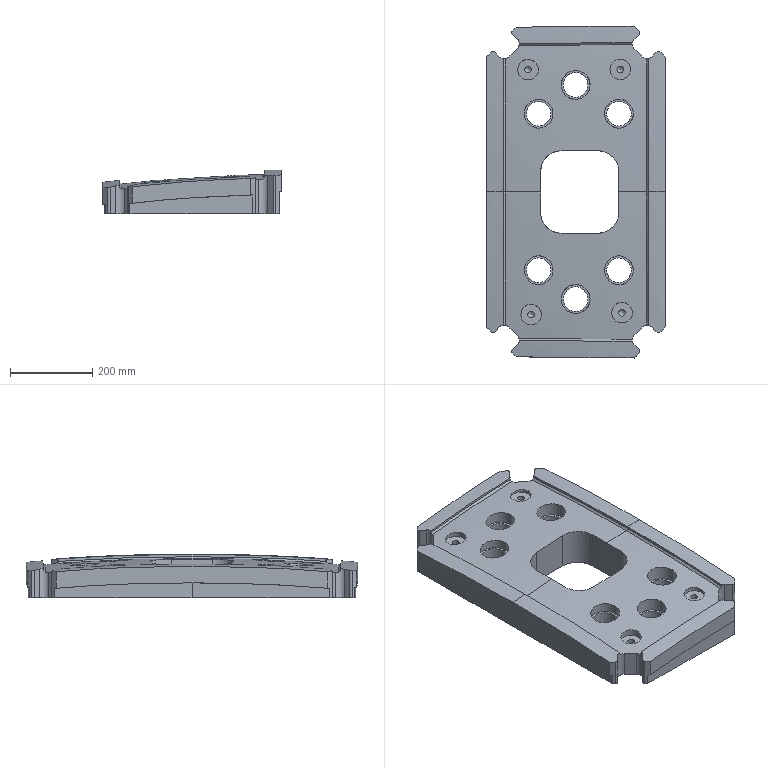Part | NX | features solid 2 | 1 solid | 113 faces | box 433.369 x 805.986 x 106.352 mm | volume 22025386 mm3 | cylinder 40 | plane 35 | spline 34 | cone 4 | commonest cylinder face diameters 10 x8 31 x8 60 x6 70 x6 16 x4 50 x4